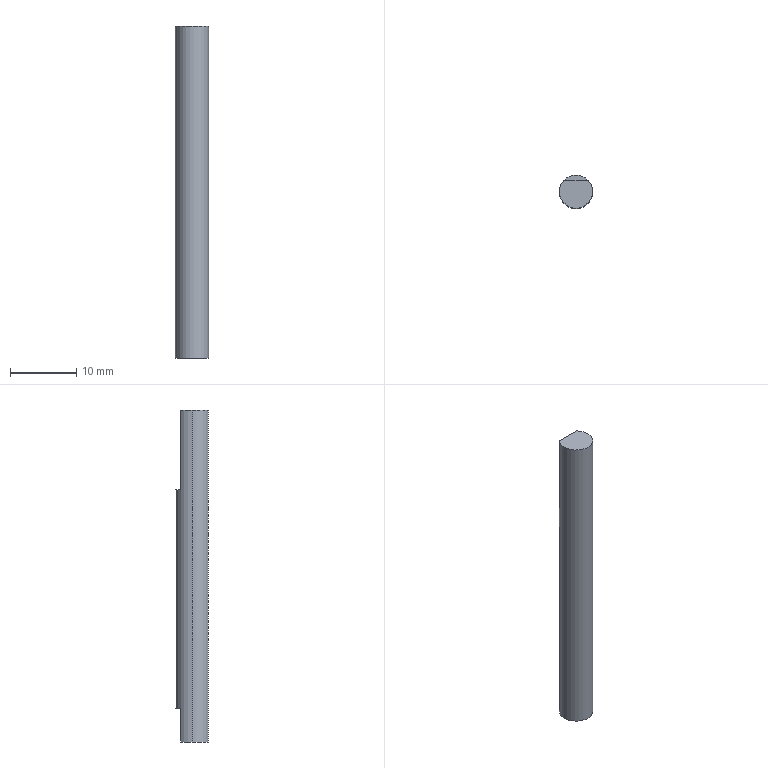Part | SolidWorks | features ICE 2, Extrusion 1 | 1 solid | 8 faces | box 5 x 5 x 50 mm | volume 947.142 mm3 | plane 6 | cylinder 2 | commonest cylinder face diameters 5 x2
STEP:
#1=CARTESIAN_POINT('',(2.5,0.,50.));
#2=VERTEX_POINT('',#1);
#3=CARTESIAN_POINT('',(1.835,1.698,50.));
#4=VERTEX_POINT('',#3);
#5=CARTESIAN_POINT('',(0.,0.,50.));
#6=DIRECTION('',(0.,0.,1.));
#7=DIRECTION('',(1.,0.,0.));
#8=AXIS2_PLACEMENT_3D('',#5,#6,#7);
#9=CIRCLE('',#8,2.5);
#10=EDGE_CURVE('',#2,#4,#9,.T.);
#11=ORIENTED_EDGE('',*,*,#10,.F.);
#12=CARTESIAN_POINT('',(2.5,0.,0.));
#13=VERTEX_POINT('',#12);
#14=CARTESIAN_POINT('',(2.5,0.,50.));
#15=DIRECTION('',(0.,0.,-1.));
#16=VECTOR('',#15,1000.);
#17=LINE('',#14,#16);
#18=EDGE_CURVE('',#2,#13,#17,.T.);
#19=ORIENTED_EDGE('',*,*,#18,.T.);
#20=CARTESIAN_POINT('',(1.835,1.698,0.));
#21=VERTEX_POINT('',#20);
#22=CARTESIAN_POINT('',(0.,0.,0.));
#23=DIRECTION('',(0.,0.,1.));
#24=DIRECTION('',(1.,0.,0.));
#25=AXIS2_PLACEMENT_3D('',#22,#23,#24);
#26=CIRCLE('',#25,2.5);
#27=EDGE_CURVE('',#13,#21,#26,.T.);
#28=ORIENTED_EDGE('',*,*,#27,.T.);
#29=CARTESIAN_POINT('',(1.835,1.698,5.));
#30=VERTEX_POINT('',#29);
#31=CARTESIAN_POINT('',(1.835,1.698,5.));
#32=DIRECTION('',(0.,0.,-1.));
#33=VECTOR('',#32,1000.);
#34=LINE('',#31,#33);
#35=EDGE_CURVE('',#30,#21,#34,.T.);
#36=ORIENTED_EDGE('',*,*,#35,.F.);
#37=CARTESIAN_POINT('',(-1.835,1.698,5.));
#38=VERTEX_POINT('',#37);
#39=CARTESIAN_POINT('',(0.,0.,5.));
#40=DIRECTION('',(0.,0.,-1.));
#41=DIRECTION('',(-1.,0.,0.));
#42=AXIS2_PLACEMENT_3D('',#39,#40,#41);
#43=CIRCLE('',#42,2.5);
#44=EDGE_CURVE('',#38,#30,#43,.T.);
#45=ORIENTED_EDGE('',*,*,#44,.F.);
#46=CARTESIAN_POINT('',(-1.835,1.698,0.));
#47=VERTEX_POINT('',#46);
#48=CARTESIAN_POINT('',(-1.835,1.698,5.));
#49=DIRECTION('',(0.,0.,-1.));
#50=VECTOR('',#49,1000.);
#51=LINE('',#48,#50);
#52=EDGE_CURVE('',#38,#47,#51,.T.);
#53=ORIENTED_EDGE('',*,*,#52,.T.);
#54=CARTESIAN_POINT('',(-2.5,0.,0.));
#55=VERTEX_POINT('',#54);
#56=CARTESIAN_POINT('',(0.,0.,0.));
#57=DIRECTION('',(0.,0.,1.));
#58=DIRECTION('',(1.,0.,0.));
#59=AXIS2_PLACEMENT_3D('',#56,#57,#58);
#60=CIRCLE('',#59,2.5);
#61=EDGE_CURVE('',#47,#55,#60,.T.);
#62=ORIENTED_EDGE('',*,*,#61,.T.);
#63=CARTESIAN_POINT('',(-2.5,0.,50.));
#64=VERTEX_POINT('',#63);
#65=CARTESIAN_POINT('',(-2.5,0.,50.));
#66=DIRECTION('',(0.,0.,-1.));
#67=VECTOR('',#66,1000.);
#68=LINE('',#65,#67);
#69=EDGE_CURVE('',#64,#55,#68,.T.);
#70=ORIENTED_EDGE('',*,*,#69,.F.);
#71=CARTESIAN_POINT('',(-1.835,1.698,50.));
#72=VERTEX_POINT('',#71);
#73=CARTESIAN_POINT('',(0.,0.,50.));
#74=DIRECTION('',(0.,0.,1.));
#75=DIRECTION('',(1.,0.,0.));
#76=AXIS2_PLACEMENT_3D('',#73,#74,#75);
#77=CIRCLE('',#76,2.5);
#78=EDGE_CURVE('',#72,#64,#77,.T.);
#79=ORIENTED_EDGE('',*,*,#78,.F.);
#80=CARTESIAN_POINT('',(-1.835,1.698,38.));
#81=VERTEX_POINT('',#80);
#82=CARTESIAN_POINT('',(-1.835,1.698,38.));
#83=DIRECTION('',(0.,0.,1.));
#84=VECTOR('',#83,1000.);
#85=LINE('',#82,#84);
#86=EDGE_CURVE('',#81,#72,#85,.T.);
#87=ORIENTED_EDGE('',*,*,#86,.F.);
#88=CARTESIAN_POINT('',(1.835,1.698,38.));
#89=VERTEX_POINT('',#88);
#90=CARTESIAN_POINT('',(0.,0.,38.));
#91=DIRECTION('',(0.,0.,1.));
#92=DIRECTION('',(1.,0.,0.));
#93=AXIS2_PLACEMENT_3D('',#90,#91,#92);
#94=CIRCLE('',#93,2.5);
#95=EDGE_CURVE('',#89,#81,#94,.T.);
#96=ORIENTED_EDGE('',*,*,#95,.F.);
#97=CARTESIAN_POINT('',(1.835,1.698,38.));
#98=DIRECTION('',(0.,0.,1.));
#99=VECTOR('',#98,1000.);
#100=LINE('',#97,#99);
#101=EDGE_CURVE('',#89,#4,#100,.T.);
#102=ORIENTED_EDGE('',*,*,#101,.T.);
#103=EDGE_LOOP('',(#11,#19,#28,#36,#45,#53,#62,#70,#79,#87,#96,#102));
#104=FACE_OUTER_BOUND('',#103,.T.);
#105=CARTESIAN_POINT('',(0.,0.,50.));
#106=DIRECTION('',(0.,0.,-1.));
#107=DIRECTION('',(-1.,0.,0.));
#108=AXIS2_PLACEMENT_3D('',#105,#106,#107);
#109=CYLINDRICAL_SURFACE('',#108,2.5);
#110=ADVANCED_FACE('',(#104),#109,.T.);
#111=ORIENTED_EDGE('',*,*,#18,.F.);
#112=CARTESIAN_POINT('',(0.,0.,50.));
#113=DIRECTION('',(0.,0.,1.));
#114=DIRECTION('',(1.,0.,0.));
#115=AXIS2_PLACEMENT_3D('',#112,#113,#114);
#116=CIRCLE('',#115,2.5);
#117=EDGE_CURVE('',#64,#2,#116,.T.);
#118=ORIENTED_EDGE('',*,*,#117,.F.);
#119=ORIENTED_EDGE('',*,*,#69,.T.);
#120=CARTESIAN_POINT('',(0.,0.,0.));
#121=DIRECTION('',(0.,0.,1.));
#122=DIRECTION('',(1.,0.,0.));
#123=AXIS2_PLACEMENT_3D('',#120,#121,#122);
#124=CIRCLE('',#123,2.5);
#125=EDGE_CURVE('',#55,#13,#124,.T.);
#126=ORIENTED_EDGE('',*,*,#125,.T.);
#127=EDGE_LOOP('',(#111,#118,#119,#126));
#128=FACE_OUTER_BOUND('',#127,.T.);
#129=CARTESIAN_POINT('',(0.,0.,50.));
#130=DIRECTION('',(0.,0.,-1.));
#131=DIRECTION('',(-1.,0.,0.));
#132=AXIS2_PLACEMENT_3D('',#129,#130,#131);
#133=CYLINDRICAL_SURFACE('',#132,2.5);
#134=ADVANCED_FACE('',(#128),#133,.T.);
#135=CARTESIAN_POINT('',(-1.835,1.698,50.));
#136=DIRECTION('',(1.,0.,0.));
#137=VECTOR('',#136,1000.);
#138=LINE('',#135,#137);
#139=EDGE_CURVE('',#72,#4,#138,.T.);
#140=ORIENTED_EDGE('',*,*,#139,.F.);
#141=ORIENTED_EDGE('',*,*,#78,.T.);
#142=ORIENTED_EDGE('',*,*,#117,.T.);
#143=ORIENTED_EDGE('',*,*,#10,.T.);
#144=EDGE_LOOP('',(#140,#141,#142,#143));
#145=FACE_OUTER_BOUND('',#144,.T.);
#146=CARTESIAN_POINT('',(0.,0.,50.));
#147=DIRECTION('',(0.,0.,1.));
#148=DIRECTION('',(1.,0.,0.));
#149=AXIS2_PLACEMENT_3D('',#146,#147,#148);
#150=PLANE('',#149);
#151=ADVANCED_FACE('',(#145),#150,.T.);
#152=ORIENTED_EDGE('',*,*,#61,.F.);
#153=CARTESIAN_POINT('',(1.835,1.698,0.));
#154=DIRECTION('',(-1.,0.,0.));
#155=VECTOR('',#154,1000.);
#156=LINE('',#153,#155);
#157=EDGE_CURVE('',#21,#47,#156,.T.);
#158=ORIENTED_EDGE('',*,*,#157,.F.);
#159=ORIENTED_EDGE('',*,*,#27,.F.);
#160=ORIENTED_EDGE('',*,*,#125,.F.);
#161=EDGE_LOOP('',(#152,#158,#159,#160));
#162=FACE_OUTER_BOUND('',#161,.T.);
#163=CARTESIAN_POINT('',(0.,0.,0.));
#164=DIRECTION('',(0.,0.,1.));
#165=DIRECTION('',(1.,0.,0.));
#166=AXIS2_PLACEMENT_3D('',#163,#164,#165);
#167=PLANE('',#166);
#168=ADVANCED_FACE('',(#162),#167,.F.);
#169=ORIENTED_EDGE('',*,*,#157,.T.);
#170=ORIENTED_EDGE('',*,*,#52,.F.);
#171=CARTESIAN_POINT('',(1.835,1.698,5.));
#172=DIRECTION('',(-1.,0.,0.));
#173=VECTOR('',#172,1000.);
#174=LINE('',#171,#173);
#175=EDGE_CURVE('',#30,#38,#174,.T.);
#176=ORIENTED_EDGE('',*,*,#175,.F.);
#177=ORIENTED_EDGE('',*,*,#35,.T.);
#178=EDGE_LOOP('',(#169,#170,#176,#177));
#179=FACE_OUTER_BOUND('',#178,.T.);
#180=CARTESIAN_POINT('',(1.835,1.698,5.));
#181=DIRECTION('',(0.,-1.,0.));
#182=DIRECTION('',(0.,0.,-1.));
#183=AXIS2_PLACEMENT_3D('',#180,#181,#182);
#184=PLANE('',#183);
#185=ADVANCED_FACE('',(#179),#184,.F.);
#186=ORIENTED_EDGE('',*,*,#44,.T.);
#187=ORIENTED_EDGE('',*,*,#175,.T.);
#188=EDGE_LOOP('',(#186,#187));
#189=FACE_OUTER_BOUND('',#188,.T.);
#190=CARTESIAN_POINT('',(0.,0.,5.));
#191=DIRECTION('',(0.,0.,-1.));
#192=DIRECTION('',(-1.,0.,0.));
#193=AXIS2_PLACEMENT_3D('',#190,#191,#192);
#194=PLANE('',#193);
#195=ADVANCED_FACE('',(#189),#194,.T.);
#196=ORIENTED_EDGE('',*,*,#139,.T.);
#197=ORIENTED_EDGE('',*,*,#101,.F.);
#198=CARTESIAN_POINT('',(-1.835,1.698,38.));
#199=DIRECTION('',(1.,0.,0.));
#200=VECTOR('',#199,1000.);
#201=LINE('',#198,#200);
#202=EDGE_CURVE('',#81,#89,#201,.T.);
#203=ORIENTED_EDGE('',*,*,#202,.F.);
#204=ORIENTED_EDGE('',*,*,#86,.T.);
#205=EDGE_LOOP('',(#196,#197,#203,#204));
#206=FACE_OUTER_BOUND('',#205,.T.);
#207=CARTESIAN_POINT('',(-1.835,1.698,38.));
#208=DIRECTION('',(0.,-1.,0.));
#209=DIRECTION('',(0.,0.,-1.));
#210=AXIS2_PLACEMENT_3D('',#207,#208,#209);
#211=PLANE('',#210);
#212=ADVANCED_FACE('',(#206),#211,.F.);
#213=ORIENTED_EDGE('',*,*,#95,.T.);
#214=ORIENTED_EDGE('',*,*,#202,.T.);
#215=EDGE_LOOP('',(#213,#214));
#216=FACE_OUTER_BOUND('',#215,.T.);
#217=CARTESIAN_POINT('',(0.,0.,38.));
#218=DIRECTION('',(0.,0.,1.));
#219=DIRECTION('',(1.,0.,0.));
#220=AXIS2_PLACEMENT_3D('',#217,#218,#219);
#221=PLANE('',#220);
#222=ADVANCED_FACE('',(#216),#221,.T.);
#223=CLOSED_SHELL('',(#110,#134,#151,#168,#185,#195,#212,#222));
#224=MANIFOLD_SOLID_BREP('',#223);
#225=CARTESIAN_POINT('',(0.,0.,0.));
#226=DIRECTION('',(0.,0.,1.));
#227=DIRECTION('',(1.,0.,0.));
#228=AXIS2_PLACEMENT_3D('',#225,#226,#227);
#229=(LENGTH_UNIT()NAMED_UNIT(*)SI_UNIT(.MILLI.,.METRE.));
#230=UNCERTAINTY_MEASURE_WITH_UNIT(LENGTH_MEASURE(0.00001),#229,'','');
#231=(NAMED_UNIT(*)PLANE_ANGLE_UNIT()SI_UNIT($,.RADIAN.));
#232=(NAMED_UNIT(*)SI_UNIT($,.STERADIAN.)SOLID_ANGLE_UNIT());
#233=(GEOMETRIC_REPRESENTATION_CONTEXT(3)GLOBAL_UNCERTAINTY_ASSIGNED_CONTEXT((#230))GLOBAL_UNIT_ASSIGNED_CONTEXT((#229,#231,#232))REPRESENTATION_CONTEXT('',''));
#234=ADVANCED_BREP_SHAPE_REPRESENTATION('',(#224,#228),#233);